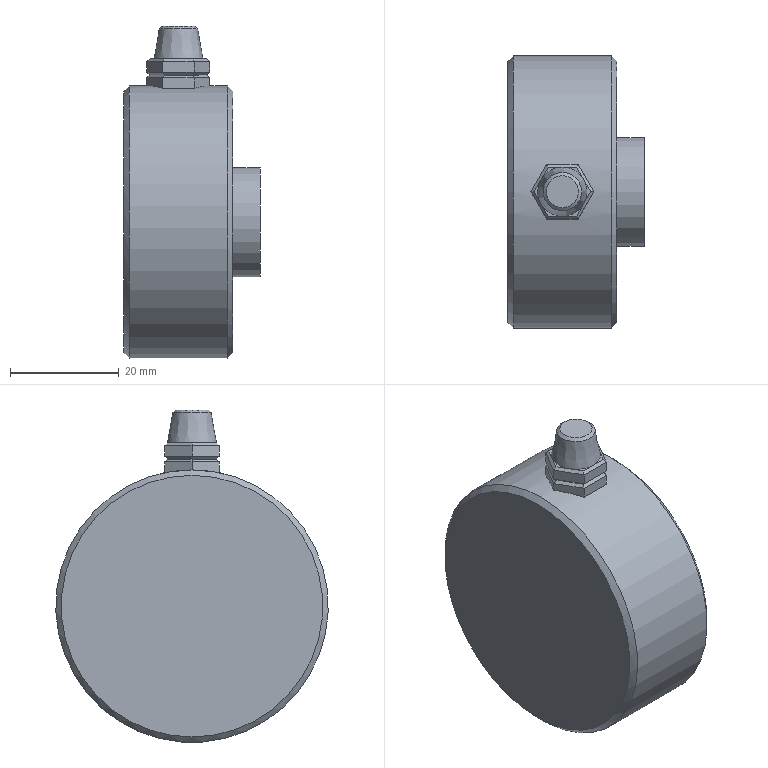Part | STEP file | Tube feed_id582_x_t | 1 solid | 52 faces | box 25 x 50 x 61 mm | volume 41415 mm3 | plane 46 | cone 4 | cylinder 2 | commonest cylinder face diameters 20 x1 50 x1